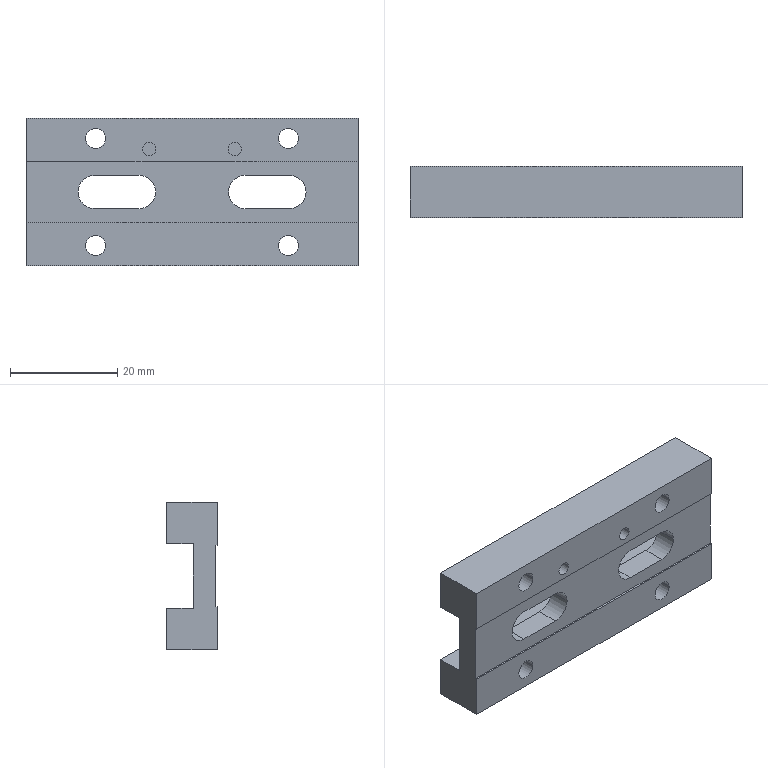Part | SolidWorks | 1 solid | 58 faces | box 62 x 9.5 x 27.6 mm | volume 10978 mm3 | cylinder 26 | plane 24 | cone 8 | commonest cylinder face diameters 3.7 x8 5.6 x8 6.2 x6 2.5 x4